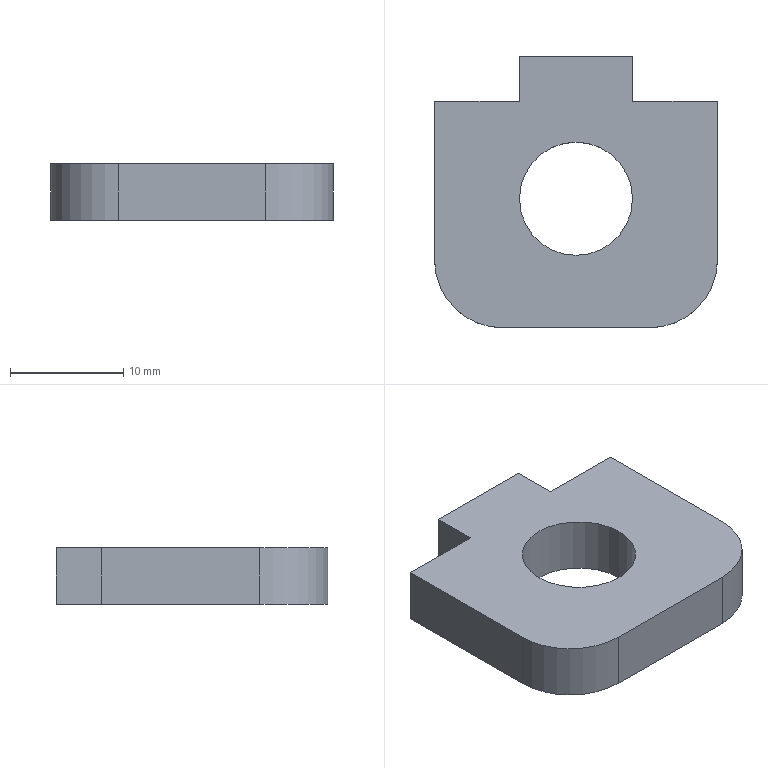Part | SolidWorks | features FlatPattern 1, SMBaseFlange 1, SheetMetal 1 | 1 solid | 14 faces | box 25 x 24 x 5 mm | volume 2230 mm3 | plane 10 | cylinder 4 | commonest cylinder face diameters 10 x2 12 x2
STEP:
#1=CARTESIAN_POINT('',(-5.,0.,5.));
#2=VERTEX_POINT('',#1);
#3=CARTESIAN_POINT('',(5.,0.,5.));
#4=VERTEX_POINT('',#3);
#5=CARTESIAN_POINT('',(0.,0.,5.));
#6=DIRECTION('',(0.,0.,1.));
#7=DIRECTION('',(1.,0.,0.));
#8=AXIS2_PLACEMENT_3D('',#5,#6,#7);
#9=CIRCLE('',#8,5.);
#10=EDGE_CURVE('',#2,#4,#9,.T.);
#11=ORIENTED_EDGE('',*,*,#10,.T.);
#12=CARTESIAN_POINT('',(5.,0.,0.));
#13=VERTEX_POINT('',#12);
#14=CARTESIAN_POINT('',(5.,0.,5.));
#15=DIRECTION('',(0.,0.,-1.));
#16=VECTOR('',#15,1000.);
#17=LINE('',#14,#16);
#18=EDGE_CURVE('',#4,#13,#17,.T.);
#19=ORIENTED_EDGE('',*,*,#18,.T.);
#20=CARTESIAN_POINT('',(-5.,0.,0.));
#21=VERTEX_POINT('',#20);
#22=CARTESIAN_POINT('',(0.,0.,0.));
#23=DIRECTION('',(0.,0.,1.));
#24=DIRECTION('',(1.,0.,0.));
#25=AXIS2_PLACEMENT_3D('',#22,#23,#24);
#26=CIRCLE('',#25,5.);
#27=EDGE_CURVE('',#21,#13,#26,.T.);
#28=ORIENTED_EDGE('',*,*,#27,.F.);
#29=CARTESIAN_POINT('',(-5.,0.,5.));
#30=DIRECTION('',(0.,0.,-1.));
#31=VECTOR('',#30,1000.);
#32=LINE('',#29,#31);
#33=EDGE_CURVE('',#2,#21,#32,.T.);
#34=ORIENTED_EDGE('',*,*,#33,.F.);
#35=EDGE_LOOP('',(#11,#19,#28,#34));
#36=FACE_OUTER_BOUND('',#35,.T.);
#37=CARTESIAN_POINT('',(0.,0.,5.));
#38=DIRECTION('',(0.,0.,-1.));
#39=DIRECTION('',(-1.,0.,0.));
#40=AXIS2_PLACEMENT_3D('',#37,#38,#39);
#41=CYLINDRICAL_SURFACE('',#40,5.);
#42=ADVANCED_FACE('',(#36),#41,.F.);
#43=CARTESIAN_POINT('',(-5.,8.6,5.));
#44=VERTEX_POINT('',#43);
#45=CARTESIAN_POINT('',(-12.5,8.6,5.));
#46=VERTEX_POINT('',#45);
#47=CARTESIAN_POINT('',(-5.,8.6,5.));
#48=DIRECTION('',(-1.,0.,0.));
#49=VECTOR('',#48,1000.);
#50=LINE('',#47,#49);
#51=EDGE_CURVE('',#44,#46,#50,.T.);
#52=ORIENTED_EDGE('',*,*,#51,.T.);
#53=CARTESIAN_POINT('',(-12.5,-5.4,5.));
#54=VERTEX_POINT('',#53);
#55=CARTESIAN_POINT('',(-12.5,-5.4,5.));
#56=DIRECTION('',(0.,-1.,0.));
#57=VECTOR('',#56,1000.);
#58=LINE('',#55,#57);
#59=EDGE_CURVE('',#46,#54,#58,.T.);
#60=ORIENTED_EDGE('',*,*,#59,.T.);
#61=CARTESIAN_POINT('',(-6.5,-11.4,5.));
#62=VERTEX_POINT('',#61);
#63=CARTESIAN_POINT('',(-6.5,-5.4,5.));
#64=DIRECTION('',(0.,0.,1.));
#65=DIRECTION('',(-1.,0.,0.));
#66=AXIS2_PLACEMENT_3D('',#63,#64,#65);
#67=CIRCLE('',#66,6.);
#68=EDGE_CURVE('',#54,#62,#67,.T.);
#69=ORIENTED_EDGE('',*,*,#68,.T.);
#70=CARTESIAN_POINT('',(6.5,-11.4,5.));
#71=VERTEX_POINT('',#70);
#72=CARTESIAN_POINT('',(6.5,-11.4,5.));
#73=DIRECTION('',(1.,0.,0.));
#74=VECTOR('',#73,1000.);
#75=LINE('',#72,#74);
#76=EDGE_CURVE('',#62,#71,#75,.T.);
#77=ORIENTED_EDGE('',*,*,#76,.T.);
#78=CARTESIAN_POINT('',(12.5,-5.4,5.));
#79=VERTEX_POINT('',#78);
#80=CARTESIAN_POINT('',(6.5,-5.4,5.));
#81=DIRECTION('',(0.,0.,1.));
#82=DIRECTION('',(1.,0.,0.));
#83=AXIS2_PLACEMENT_3D('',#80,#81,#82);
#84=CIRCLE('',#83,6.);
#85=EDGE_CURVE('',#71,#79,#84,.T.);
#86=ORIENTED_EDGE('',*,*,#85,.T.);
#87=CARTESIAN_POINT('',(12.5,8.6,5.));
#88=VERTEX_POINT('',#87);
#89=CARTESIAN_POINT('',(12.5,-5.4,5.));
#90=DIRECTION('',(0.,1.,0.));
#91=VECTOR('',#90,1000.);
#92=LINE('',#89,#91);
#93=EDGE_CURVE('',#79,#88,#92,.T.);
#94=ORIENTED_EDGE('',*,*,#93,.T.);
#95=CARTESIAN_POINT('',(5.,8.6,5.));
#96=VERTEX_POINT('',#95);
#97=CARTESIAN_POINT('',(12.5,8.6,5.));
#98=DIRECTION('',(-1.,0.,0.));
#99=VECTOR('',#98,1000.);
#100=LINE('',#97,#99);
#101=EDGE_CURVE('',#88,#96,#100,.T.);
#102=ORIENTED_EDGE('',*,*,#101,.T.);
#103=CARTESIAN_POINT('',(5.,12.6,5.));
#104=VERTEX_POINT('',#103);
#105=CARTESIAN_POINT('',(5.,8.6,5.));
#106=DIRECTION('',(0.,1.,0.));
#107=VECTOR('',#106,1000.);
#108=LINE('',#105,#107);
#109=EDGE_CURVE('',#96,#104,#108,.T.);
#110=ORIENTED_EDGE('',*,*,#109,.T.);
#111=CARTESIAN_POINT('',(-5.,12.6,5.));
#112=VERTEX_POINT('',#111);
#113=CARTESIAN_POINT('',(5.,12.6,5.));
#114=DIRECTION('',(-1.,0.,0.));
#115=VECTOR('',#114,1000.);
#116=LINE('',#113,#115);
#117=EDGE_CURVE('',#104,#112,#116,.T.);
#118=ORIENTED_EDGE('',*,*,#117,.T.);
#119=CARTESIAN_POINT('',(-5.,12.6,5.));
#120=DIRECTION('',(0.,-1.,0.));
#121=VECTOR('',#120,1000.);
#122=LINE('',#119,#121);
#123=EDGE_CURVE('',#112,#44,#122,.T.);
#124=ORIENTED_EDGE('',*,*,#123,.T.);
#125=EDGE_LOOP('',(#52,#60,#69,#77,#86,#94,#102,#110,#118,#124));
#126=FACE_OUTER_BOUND('',#125,.T.);
#127=ORIENTED_EDGE('',*,*,#10,.F.);
#128=CARTESIAN_POINT('',(0.,0.,5.));
#129=DIRECTION('',(0.,0.,1.));
#130=DIRECTION('',(1.,0.,0.));
#131=AXIS2_PLACEMENT_3D('',#128,#129,#130);
#132=CIRCLE('',#131,5.);
#133=EDGE_CURVE('',#4,#2,#132,.T.);
#134=ORIENTED_EDGE('',*,*,#133,.F.);
#135=EDGE_LOOP('',(#127,#134));
#136=FACE_BOUND('',#135,.T.);
#137=CARTESIAN_POINT('',(-6.5,-5.4,5.));
#138=DIRECTION('',(0.,0.,-1.));
#139=DIRECTION('',(-1.,0.,0.));
#140=AXIS2_PLACEMENT_3D('',#137,#138,#139);
#141=PLANE('',#140);
#142=ADVANCED_FACE('',(#126,#136),#141,.F.);
#143=CARTESIAN_POINT('',(-5.,8.6,0.));
#144=VERTEX_POINT('',#143);
#145=CARTESIAN_POINT('',(-12.5,8.6,0.));
#146=VERTEX_POINT('',#145);
#147=CARTESIAN_POINT('',(-5.,8.6,0.));
#148=DIRECTION('',(-1.,0.,0.));
#149=VECTOR('',#148,1000.);
#150=LINE('',#147,#149);
#151=EDGE_CURVE('',#144,#146,#150,.T.);
#152=ORIENTED_EDGE('',*,*,#151,.F.);
#153=CARTESIAN_POINT('',(-5.,12.6,0.));
#154=VERTEX_POINT('',#153);
#155=CARTESIAN_POINT('',(-5.,12.6,0.));
#156=DIRECTION('',(0.,-1.,0.));
#157=VECTOR('',#156,1000.);
#158=LINE('',#155,#157);
#159=EDGE_CURVE('',#154,#144,#158,.T.);
#160=ORIENTED_EDGE('',*,*,#159,.F.);
#161=CARTESIAN_POINT('',(5.,12.6,0.));
#162=VERTEX_POINT('',#161);
#163=CARTESIAN_POINT('',(5.,12.6,0.));
#164=DIRECTION('',(-1.,0.,0.));
#165=VECTOR('',#164,1000.);
#166=LINE('',#163,#165);
#167=EDGE_CURVE('',#162,#154,#166,.T.);
#168=ORIENTED_EDGE('',*,*,#167,.F.);
#169=CARTESIAN_POINT('',(5.,8.6,0.));
#170=VERTEX_POINT('',#169);
#171=CARTESIAN_POINT('',(5.,8.6,0.));
#172=DIRECTION('',(0.,1.,0.));
#173=VECTOR('',#172,1000.);
#174=LINE('',#171,#173);
#175=EDGE_CURVE('',#170,#162,#174,.T.);
#176=ORIENTED_EDGE('',*,*,#175,.F.);
#177=CARTESIAN_POINT('',(12.5,8.6,0.));
#178=VERTEX_POINT('',#177);
#179=CARTESIAN_POINT('',(12.5,8.6,0.));
#180=DIRECTION('',(-1.,0.,0.));
#181=VECTOR('',#180,1000.);
#182=LINE('',#179,#181);
#183=EDGE_CURVE('',#178,#170,#182,.T.);
#184=ORIENTED_EDGE('',*,*,#183,.F.);
#185=CARTESIAN_POINT('',(12.5,-5.4,0.));
#186=VERTEX_POINT('',#185);
#187=CARTESIAN_POINT('',(12.5,-5.4,0.));
#188=DIRECTION('',(0.,1.,0.));
#189=VECTOR('',#188,1000.);
#190=LINE('',#187,#189);
#191=EDGE_CURVE('',#186,#178,#190,.T.);
#192=ORIENTED_EDGE('',*,*,#191,.F.);
#193=CARTESIAN_POINT('',(6.5,-11.4,0.));
#194=VERTEX_POINT('',#193);
#195=CARTESIAN_POINT('',(6.5,-5.4,0.));
#196=DIRECTION('',(0.,0.,1.));
#197=DIRECTION('',(1.,0.,0.));
#198=AXIS2_PLACEMENT_3D('',#195,#196,#197);
#199=CIRCLE('',#198,6.);
#200=EDGE_CURVE('',#194,#186,#199,.T.);
#201=ORIENTED_EDGE('',*,*,#200,.F.);
#202=CARTESIAN_POINT('',(-6.5,-11.4,0.));
#203=VERTEX_POINT('',#202);
#204=CARTESIAN_POINT('',(6.5,-11.4,0.));
#205=DIRECTION('',(1.,0.,0.));
#206=VECTOR('',#205,1000.);
#207=LINE('',#204,#206);
#208=EDGE_CURVE('',#203,#194,#207,.T.);
#209=ORIENTED_EDGE('',*,*,#208,.F.);
#210=CARTESIAN_POINT('',(-12.5,-5.4,0.));
#211=VERTEX_POINT('',#210);
#212=CARTESIAN_POINT('',(-6.5,-5.4,0.));
#213=DIRECTION('',(0.,0.,1.));
#214=DIRECTION('',(-1.,0.,0.));
#215=AXIS2_PLACEMENT_3D('',#212,#213,#214);
#216=CIRCLE('',#215,6.);
#217=EDGE_CURVE('',#211,#203,#216,.T.);
#218=ORIENTED_EDGE('',*,*,#217,.F.);
#219=CARTESIAN_POINT('',(-12.5,-5.4,0.));
#220=DIRECTION('',(0.,-1.,0.));
#221=VECTOR('',#220,1000.);
#222=LINE('',#219,#221);
#223=EDGE_CURVE('',#146,#211,#222,.T.);
#224=ORIENTED_EDGE('',*,*,#223,.F.);
#225=EDGE_LOOP('',(#152,#160,#168,#176,#184,#192,#201,#209,#218,#224));
#226=FACE_OUTER_BOUND('',#225,.T.);
#227=ORIENTED_EDGE('',*,*,#27,.T.);
#228=CARTESIAN_POINT('',(0.,0.,0.));
#229=DIRECTION('',(0.,0.,1.));
#230=DIRECTION('',(1.,0.,0.));
#231=AXIS2_PLACEMENT_3D('',#228,#229,#230);
#232=CIRCLE('',#231,5.);
#233=EDGE_CURVE('',#13,#21,#232,.T.);
#234=ORIENTED_EDGE('',*,*,#233,.T.);
#235=EDGE_LOOP('',(#227,#234));
#236=FACE_BOUND('',#235,.T.);
#237=CARTESIAN_POINT('',(-6.5,-5.4,0.));
#238=DIRECTION('',(0.,0.,-1.));
#239=DIRECTION('',(-1.,0.,0.));
#240=AXIS2_PLACEMENT_3D('',#237,#238,#239);
#241=PLANE('',#240);
#242=ADVANCED_FACE('',(#226,#236),#241,.T.);
#243=ORIENTED_EDGE('',*,*,#151,.T.);
#244=CARTESIAN_POINT('',(-12.5,8.6,5.));
#245=DIRECTION('',(0.,0.,-1.));
#246=VECTOR('',#245,1000.);
#247=LINE('',#244,#246);
#248=EDGE_CURVE('',#46,#146,#247,.T.);
#249=ORIENTED_EDGE('',*,*,#248,.F.);
#250=ORIENTED_EDGE('',*,*,#51,.F.);
#251=CARTESIAN_POINT('',(-5.,8.6,5.));
#252=DIRECTION('',(0.,0.,-1.));
#253=VECTOR('',#252,1000.);
#254=LINE('',#251,#253);
#255=EDGE_CURVE('',#44,#144,#254,.T.);
#256=ORIENTED_EDGE('',*,*,#255,.T.);
#257=EDGE_LOOP('',(#243,#249,#250,#256));
#258=FACE_OUTER_BOUND('',#257,.T.);
#259=CARTESIAN_POINT('',(-5.,8.6,5.));
#260=DIRECTION('',(0.,-1.,0.));
#261=DIRECTION('',(1.,0.,0.));
#262=AXIS2_PLACEMENT_3D('',#259,#260,#261);
#263=PLANE('',#262);
#264=ADVANCED_FACE('',(#258),#263,.F.);
#265=ORIENTED_EDGE('',*,*,#223,.T.);
#266=CARTESIAN_POINT('',(-12.5,-5.4,5.));
#267=DIRECTION('',(0.,0.,-1.));
#268=VECTOR('',#267,1000.);
#269=LINE('',#266,#268);
#270=EDGE_CURVE('',#54,#211,#269,.T.);
#271=ORIENTED_EDGE('',*,*,#270,.F.);
#272=ORIENTED_EDGE('',*,*,#59,.F.);
#273=ORIENTED_EDGE('',*,*,#248,.T.);
#274=EDGE_LOOP('',(#265,#271,#272,#273));
#275=FACE_OUTER_BOUND('',#274,.T.);
#276=CARTESIAN_POINT('',(-12.5,-5.4,5.));
#277=DIRECTION('',(1.,0.,0.));
#278=DIRECTION('',(0.,1.,0.));
#279=AXIS2_PLACEMENT_3D('',#276,#277,#278);
#280=PLANE('',#279);
#281=ADVANCED_FACE('',(#275),#280,.F.);
#282=ORIENTED_EDGE('',*,*,#217,.T.);
#283=CARTESIAN_POINT('',(-6.5,-11.4,5.));
#284=DIRECTION('',(0.,0.,-1.));
#285=VECTOR('',#284,1000.);
#286=LINE('',#283,#285);
#287=EDGE_CURVE('',#62,#203,#286,.T.);
#288=ORIENTED_EDGE('',*,*,#287,.F.);
#289=ORIENTED_EDGE('',*,*,#68,.F.);
#290=ORIENTED_EDGE('',*,*,#270,.T.);
#291=EDGE_LOOP('',(#282,#288,#289,#290));
#292=FACE_OUTER_BOUND('',#291,.T.);
#293=CARTESIAN_POINT('',(-6.5,-5.4,5.));
#294=DIRECTION('',(0.,0.,-1.));
#295=DIRECTION('',(-1.,0.,0.));
#296=AXIS2_PLACEMENT_3D('',#293,#294,#295);
#297=CYLINDRICAL_SURFACE('',#296,6.);
#298=ADVANCED_FACE('',(#292),#297,.T.);
#299=ORIENTED_EDGE('',*,*,#208,.T.);
#300=CARTESIAN_POINT('',(6.5,-11.4,5.));
#301=DIRECTION('',(0.,0.,-1.));
#302=VECTOR('',#301,1000.);
#303=LINE('',#300,#302);
#304=EDGE_CURVE('',#71,#194,#303,.T.);
#305=ORIENTED_EDGE('',*,*,#304,.F.);
#306=ORIENTED_EDGE('',*,*,#76,.F.);
#307=ORIENTED_EDGE('',*,*,#287,.T.);
#308=EDGE_LOOP('',(#299,#305,#306,#307));
#309=FACE_OUTER_BOUND('',#308,.T.);
#310=CARTESIAN_POINT('',(6.5,-11.4,5.));
#311=DIRECTION('',(0.,1.,0.));
#312=DIRECTION('',(0.,0.,1.));
#313=AXIS2_PLACEMENT_3D('',#310,#311,#312);
#314=PLANE('',#313);
#315=ADVANCED_FACE('',(#309),#314,.F.);
#316=ORIENTED_EDGE('',*,*,#200,.T.);
#317=CARTESIAN_POINT('',(12.5,-5.4,5.));
#318=DIRECTION('',(0.,0.,-1.));
#319=VECTOR('',#318,1000.);
#320=LINE('',#317,#319);
#321=EDGE_CURVE('',#79,#186,#320,.T.);
#322=ORIENTED_EDGE('',*,*,#321,.F.);
#323=ORIENTED_EDGE('',*,*,#85,.F.);
#324=ORIENTED_EDGE('',*,*,#304,.T.);
#325=EDGE_LOOP('',(#316,#322,#323,#324));
#326=FACE_OUTER_BOUND('',#325,.T.);
#327=CARTESIAN_POINT('',(6.5,-5.4,5.));
#328=DIRECTION('',(0.,0.,-1.));
#329=DIRECTION('',(-1.,0.,0.));
#330=AXIS2_PLACEMENT_3D('',#327,#328,#329);
#331=CYLINDRICAL_SURFACE('',#330,6.);
#332=ADVANCED_FACE('',(#326),#331,.T.);
#333=ORIENTED_EDGE('',*,*,#191,.T.);
#334=CARTESIAN_POINT('',(12.5,8.6,5.));
#335=DIRECTION('',(0.,0.,-1.));
#336=VECTOR('',#335,1000.);
#337=LINE('',#334,#336);
#338=EDGE_CURVE('',#88,#178,#337,.T.);
#339=ORIENTED_EDGE('',*,*,#338,.F.);
#340=ORIENTED_EDGE('',*,*,#93,.F.);
#341=ORIENTED_EDGE('',*,*,#321,.T.);
#342=EDGE_LOOP('',(#333,#339,#340,#341));
#343=FACE_OUTER_BOUND('',#342,.T.);
#344=CARTESIAN_POINT('',(12.5,-5.4,5.));
#345=DIRECTION('',(-1.,0.,0.));
#346=DIRECTION('',(0.,0.,1.));
#347=AXIS2_PLACEMENT_3D('',#344,#345,#346);
#348=PLANE('',#347);
#349=ADVANCED_FACE('',(#343),#348,.F.);
#350=ORIENTED_EDGE('',*,*,#183,.T.);
#351=CARTESIAN_POINT('',(5.,8.6,5.));
#352=DIRECTION('',(0.,0.,-1.));
#353=VECTOR('',#352,1000.);
#354=LINE('',#351,#353);
#355=EDGE_CURVE('',#96,#170,#354,.T.);
#356=ORIENTED_EDGE('',*,*,#355,.F.);
#357=ORIENTED_EDGE('',*,*,#101,.F.);
#358=ORIENTED_EDGE('',*,*,#338,.T.);
#359=EDGE_LOOP('',(#350,#356,#357,#358));
#360=FACE_OUTER_BOUND('',#359,.T.);
#361=CARTESIAN_POINT('',(12.5,8.6,5.));
#362=DIRECTION('',(0.,-1.,0.));
#363=DIRECTION('',(1.,0.,0.));
#364=AXIS2_PLACEMENT_3D('',#361,#362,#363);
#365=PLANE('',#364);
#366=ADVANCED_FACE('',(#360),#365,.F.);
#367=ORIENTED_EDGE('',*,*,#175,.T.);
#368=CARTESIAN_POINT('',(5.,12.6,5.));
#369=DIRECTION('',(0.,0.,-1.));
#370=VECTOR('',#369,1000.);
#371=LINE('',#368,#370);
#372=EDGE_CURVE('',#104,#162,#371,.T.);
#373=ORIENTED_EDGE('',*,*,#372,.F.);
#374=ORIENTED_EDGE('',*,*,#109,.F.);
#375=ORIENTED_EDGE('',*,*,#355,.T.);
#376=EDGE_LOOP('',(#367,#373,#374,#375));
#377=FACE_OUTER_BOUND('',#376,.T.);
#378=CARTESIAN_POINT('',(5.,8.6,5.));
#379=DIRECTION('',(-1.,0.,0.));
#380=DIRECTION('',(0.,0.,1.));
#381=AXIS2_PLACEMENT_3D('',#378,#379,#380);
#382=PLANE('',#381);
#383=ADVANCED_FACE('',(#377),#382,.F.);
#384=ORIENTED_EDGE('',*,*,#167,.T.);
#385=CARTESIAN_POINT('',(-5.,12.6,5.));
#386=DIRECTION('',(0.,0.,-1.));
#387=VECTOR('',#386,1000.);
#388=LINE('',#385,#387);
#389=EDGE_CURVE('',#112,#154,#388,.T.);
#390=ORIENTED_EDGE('',*,*,#389,.F.);
#391=ORIENTED_EDGE('',*,*,#117,.F.);
#392=ORIENTED_EDGE('',*,*,#372,.T.);
#393=EDGE_LOOP('',(#384,#390,#391,#392));
#394=FACE_OUTER_BOUND('',#393,.T.);
#395=CARTESIAN_POINT('',(5.,12.6,5.));
#396=DIRECTION('',(0.,-1.,0.));
#397=DIRECTION('',(1.,0.,0.));
#398=AXIS2_PLACEMENT_3D('',#395,#396,#397);
#399=PLANE('',#398);
#400=ADVANCED_FACE('',(#394),#399,.F.);
#401=ORIENTED_EDGE('',*,*,#159,.T.);
#402=ORIENTED_EDGE('',*,*,#255,.F.);
#403=ORIENTED_EDGE('',*,*,#123,.F.);
#404=ORIENTED_EDGE('',*,*,#389,.T.);
#405=EDGE_LOOP('',(#401,#402,#403,#404));
#406=FACE_OUTER_BOUND('',#405,.T.);
#407=CARTESIAN_POINT('',(-5.,12.6,5.));
#408=DIRECTION('',(1.,0.,0.));
#409=DIRECTION('',(0.,0.,-1.));
#410=AXIS2_PLACEMENT_3D('',#407,#408,#409);
#411=PLANE('',#410);
#412=ADVANCED_FACE('',(#406),#411,.F.);
#413=ORIENTED_EDGE('',*,*,#18,.F.);
#414=ORIENTED_EDGE('',*,*,#133,.T.);
#415=ORIENTED_EDGE('',*,*,#33,.T.);
#416=ORIENTED_EDGE('',*,*,#233,.F.);
#417=EDGE_LOOP('',(#413,#414,#415,#416));
#418=FACE_OUTER_BOUND('',#417,.T.);
#419=CARTESIAN_POINT('',(0.,0.,5.));
#420=DIRECTION('',(0.,0.,-1.));
#421=DIRECTION('',(-1.,0.,0.));
#422=AXIS2_PLACEMENT_3D('',#419,#420,#421);
#423=CYLINDRICAL_SURFACE('',#422,5.);
#424=ADVANCED_FACE('',(#418),#423,.F.);
#425=CLOSED_SHELL('',(#42,#142,#242,#264,#281,#298,#315,#332,#349,#366,#383,#400,#412,#424));
#426=MANIFOLD_SOLID_BREP('',#425);
#427=CARTESIAN_POINT('',(0.,0.,0.));
#428=DIRECTION('',(0.,0.,1.));
#429=DIRECTION('',(1.,0.,0.));
#430=AXIS2_PLACEMENT_3D('',#427,#428,#429);
#431=(LENGTH_UNIT()NAMED_UNIT(*)SI_UNIT(.MILLI.,.METRE.));
#432=UNCERTAINTY_MEASURE_WITH_UNIT(LENGTH_MEASURE(0.00001),#431,'','');
#433=(NAMED_UNIT(*)PLANE_ANGLE_UNIT()SI_UNIT($,.RADIAN.));
#434=(NAMED_UNIT(*)SI_UNIT($,.STERADIAN.)SOLID_ANGLE_UNIT());
#435=(GEOMETRIC_REPRESENTATION_CONTEXT(3)GLOBAL_UNCERTAINTY_ASSIGNED_CONTEXT((#432))GLOBAL_UNIT_ASSIGNED_CONTEXT((#431,#433,#434))REPRESENTATION_CONTEXT('',''));
#436=ADVANCED_BREP_SHAPE_REPRESENTATION('',(#426,#430),#435);